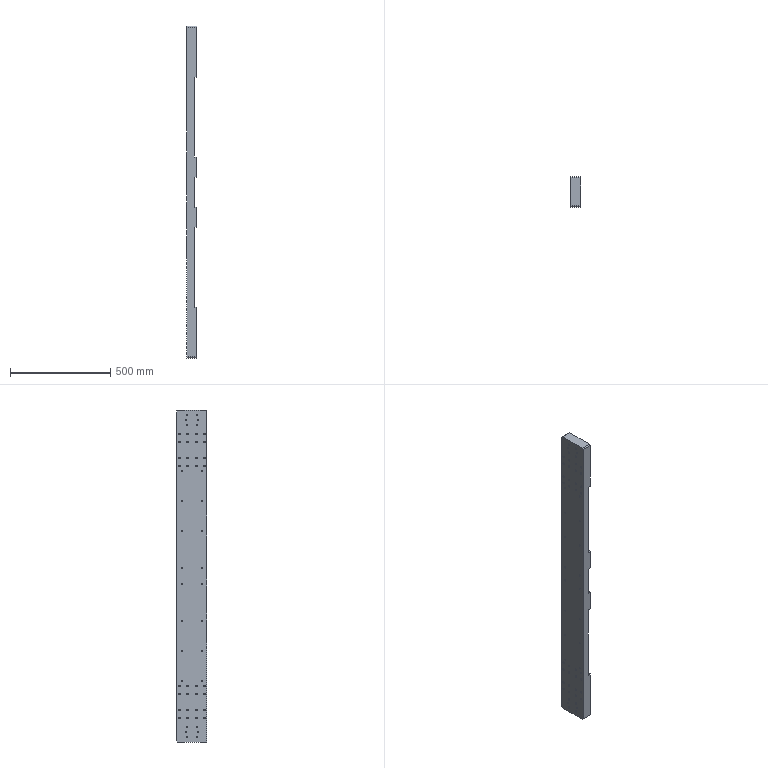Part | SolidWorks | features HoleWzd 5, MirrorPattern 4, Chamfer 1, Extrusion 1, ICE 1, LPattern 1 | 1 solid | 238 faces | box 50 x 150 x 1660 mm | volume 10088641 mm3 | cylinder 184 | plane 54 | commonest cylinder face diameters 9 x64 15 x64 6.8 x40 8.5 x16